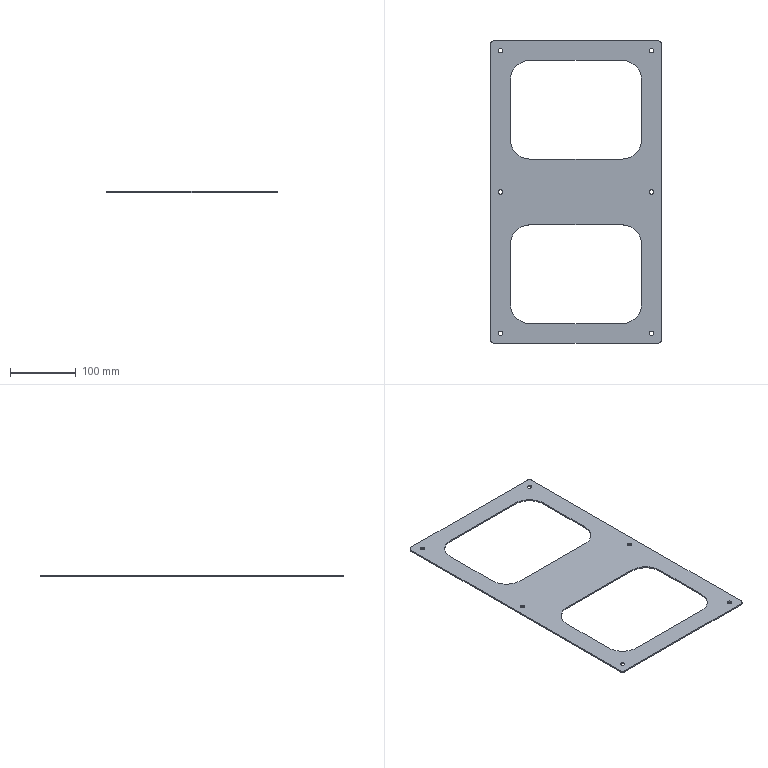Part | SolidWorks | features ICE 2, Extrusion 1, Fillet 1 | 1 solid | 38 faces | box 260 x 460 x 2 mm | volume 121786 mm3 | cylinder 24 | plane 14 | commonest cylinder face diameters 7 x12 60 x8 10 x4
STEP:
#1=CARTESIAN_POINT('',(18.5,-230.,2.));
#2=VERTEX_POINT('',#1);
#3=CARTESIAN_POINT('',(11.5,-230.,2.));
#4=VERTEX_POINT('',#3);
#5=CARTESIAN_POINT('',(15.,-230.,2.));
#6=DIRECTION('',(0.,0.,-1.));
#7=DIRECTION('',(-1.,0.,0.));
#8=AXIS2_PLACEMENT_3D('',#5,#6,#7);
#9=CIRCLE('',#8,3.5);
#10=EDGE_CURVE('',#2,#4,#9,.T.);
#11=ORIENTED_EDGE('',*,*,#10,.F.);
#12=CARTESIAN_POINT('',(18.5,-230.,0.));
#13=VERTEX_POINT('',#12);
#14=CARTESIAN_POINT('',(18.5,-230.,2.));
#15=DIRECTION('',(0.,0.,-1.));
#16=VECTOR('',#15,1000.);
#17=LINE('',#14,#16);
#18=EDGE_CURVE('',#2,#13,#17,.T.);
#19=ORIENTED_EDGE('',*,*,#18,.T.);
#20=CARTESIAN_POINT('',(11.5,-230.,0.));
#21=VERTEX_POINT('',#20);
#22=CARTESIAN_POINT('',(15.,-230.,0.));
#23=DIRECTION('',(0.,0.,-1.));
#24=DIRECTION('',(-1.,0.,0.));
#25=AXIS2_PLACEMENT_3D('',#22,#23,#24);
#26=CIRCLE('',#25,3.5);
#27=EDGE_CURVE('',#13,#21,#26,.T.);
#28=ORIENTED_EDGE('',*,*,#27,.T.);
#29=CARTESIAN_POINT('',(11.5,-230.,2.));
#30=DIRECTION('',(0.,0.,-1.));
#31=VECTOR('',#30,1000.);
#32=LINE('',#29,#31);
#33=EDGE_CURVE('',#4,#21,#32,.T.);
#34=ORIENTED_EDGE('',*,*,#33,.F.);
#35=EDGE_LOOP('',(#11,#19,#28,#34));
#36=FACE_OUTER_BOUND('',#35,.T.);
#37=CARTESIAN_POINT('',(15.,-230.,2.));
#38=DIRECTION('',(0.,0.,-1.));
#39=DIRECTION('',(-1.,0.,0.));
#40=AXIS2_PLACEMENT_3D('',#37,#38,#39);
#41=CYLINDRICAL_SURFACE('',#40,3.5);
#42=ADVANCED_FACE('',(#36),#41,.F.);
#43=CARTESIAN_POINT('',(248.5,-230.,2.));
#44=VERTEX_POINT('',#43);
#45=CARTESIAN_POINT('',(241.5,-230.,2.));
#46=VERTEX_POINT('',#45);
#47=CARTESIAN_POINT('',(245.,-230.,2.));
#48=DIRECTION('',(0.,0.,-1.));
#49=DIRECTION('',(-1.,0.,0.));
#50=AXIS2_PLACEMENT_3D('',#47,#48,#49);
#51=CIRCLE('',#50,3.5);
#52=EDGE_CURVE('',#44,#46,#51,.T.);
#53=ORIENTED_EDGE('',*,*,#52,.F.);
#54=CARTESIAN_POINT('',(248.5,-230.,0.));
#55=VERTEX_POINT('',#54);
#56=CARTESIAN_POINT('',(248.5,-230.,2.));
#57=DIRECTION('',(0.,0.,-1.));
#58=VECTOR('',#57,1000.);
#59=LINE('',#56,#58);
#60=EDGE_CURVE('',#44,#55,#59,.T.);
#61=ORIENTED_EDGE('',*,*,#60,.T.);
#62=CARTESIAN_POINT('',(241.5,-230.,0.));
#63=VERTEX_POINT('',#62);
#64=CARTESIAN_POINT('',(245.,-230.,0.));
#65=DIRECTION('',(0.,0.,-1.));
#66=DIRECTION('',(-1.,0.,0.));
#67=AXIS2_PLACEMENT_3D('',#64,#65,#66);
#68=CIRCLE('',#67,3.5);
#69=EDGE_CURVE('',#55,#63,#68,.T.);
#70=ORIENTED_EDGE('',*,*,#69,.T.);
#71=CARTESIAN_POINT('',(241.5,-230.,2.));
#72=DIRECTION('',(0.,0.,-1.));
#73=VECTOR('',#72,1000.);
#74=LINE('',#71,#73);
#75=EDGE_CURVE('',#46,#63,#74,.T.);
#76=ORIENTED_EDGE('',*,*,#75,.F.);
#77=EDGE_LOOP('',(#53,#61,#70,#76));
#78=FACE_OUTER_BOUND('',#77,.T.);
#79=CARTESIAN_POINT('',(245.,-230.,2.));
#80=DIRECTION('',(0.,0.,-1.));
#81=DIRECTION('',(-1.,0.,0.));
#82=AXIS2_PLACEMENT_3D('',#79,#80,#81);
#83=CYLINDRICAL_SURFACE('',#82,3.5);
#84=ADVANCED_FACE('',(#78),#83,.F.);
#85=CARTESIAN_POINT('',(18.5,-15.,2.));
#86=VERTEX_POINT('',#85);
#87=CARTESIAN_POINT('',(11.5,-15.,2.));
#88=VERTEX_POINT('',#87);
#89=CARTESIAN_POINT('',(15.,-15.,2.));
#90=DIRECTION('',(0.,0.,-1.));
#91=DIRECTION('',(-1.,0.,0.));
#92=AXIS2_PLACEMENT_3D('',#89,#90,#91);
#93=CIRCLE('',#92,3.5);
#94=EDGE_CURVE('',#86,#88,#93,.T.);
#95=ORIENTED_EDGE('',*,*,#94,.F.);
#96=CARTESIAN_POINT('',(18.5,-15.,0.));
#97=VERTEX_POINT('',#96);
#98=CARTESIAN_POINT('',(18.5,-15.,2.));
#99=DIRECTION('',(0.,0.,-1.));
#100=VECTOR('',#99,1000.);
#101=LINE('',#98,#100);
#102=EDGE_CURVE('',#86,#97,#101,.T.);
#103=ORIENTED_EDGE('',*,*,#102,.T.);
#104=CARTESIAN_POINT('',(11.5,-15.,0.));
#105=VERTEX_POINT('',#104);
#106=CARTESIAN_POINT('',(15.,-15.,0.));
#107=DIRECTION('',(0.,0.,-1.));
#108=DIRECTION('',(-1.,0.,0.));
#109=AXIS2_PLACEMENT_3D('',#106,#107,#108);
#110=CIRCLE('',#109,3.5);
#111=EDGE_CURVE('',#97,#105,#110,.T.);
#112=ORIENTED_EDGE('',*,*,#111,.T.);
#113=CARTESIAN_POINT('',(11.5,-15.,2.));
#114=DIRECTION('',(0.,0.,-1.));
#115=VECTOR('',#114,1000.);
#116=LINE('',#113,#115);
#117=EDGE_CURVE('',#88,#105,#116,.T.);
#118=ORIENTED_EDGE('',*,*,#117,.F.);
#119=EDGE_LOOP('',(#95,#103,#112,#118));
#120=FACE_OUTER_BOUND('',#119,.T.);
#121=CARTESIAN_POINT('',(15.,-15.,2.));
#122=DIRECTION('',(0.,0.,-1.));
#123=DIRECTION('',(-1.,0.,0.));
#124=AXIS2_PLACEMENT_3D('',#121,#122,#123);
#125=CYLINDRICAL_SURFACE('',#124,3.5);
#126=ADVANCED_FACE('',(#120),#125,.F.);
#127=CARTESIAN_POINT('',(248.5,-15.,2.));
#128=VERTEX_POINT('',#127);
#129=CARTESIAN_POINT('',(241.5,-15.,2.));
#130=VERTEX_POINT('',#129);
#131=CARTESIAN_POINT('',(245.,-15.,2.));
#132=DIRECTION('',(0.,0.,-1.));
#133=DIRECTION('',(-1.,0.,0.));
#134=AXIS2_PLACEMENT_3D('',#131,#132,#133);
#135=CIRCLE('',#134,3.5);
#136=EDGE_CURVE('',#128,#130,#135,.T.);
#137=ORIENTED_EDGE('',*,*,#136,.F.);
#138=CARTESIAN_POINT('',(248.5,-15.,0.));
#139=VERTEX_POINT('',#138);
#140=CARTESIAN_POINT('',(248.5,-15.,2.));
#141=DIRECTION('',(0.,0.,-1.));
#142=VECTOR('',#141,1000.);
#143=LINE('',#140,#142);
#144=EDGE_CURVE('',#128,#139,#143,.T.);
#145=ORIENTED_EDGE('',*,*,#144,.T.);
#146=CARTESIAN_POINT('',(241.5,-15.,0.));
#147=VERTEX_POINT('',#146);
#148=CARTESIAN_POINT('',(245.,-15.,0.));
#149=DIRECTION('',(0.,0.,-1.));
#150=DIRECTION('',(-1.,0.,0.));
#151=AXIS2_PLACEMENT_3D('',#148,#149,#150);
#152=CIRCLE('',#151,3.5);
#153=EDGE_CURVE('',#139,#147,#152,.T.);
#154=ORIENTED_EDGE('',*,*,#153,.T.);
#155=CARTESIAN_POINT('',(241.5,-15.,2.));
#156=DIRECTION('',(0.,0.,-1.));
#157=VECTOR('',#156,1000.);
#158=LINE('',#155,#157);
#159=EDGE_CURVE('',#130,#147,#158,.T.);
#160=ORIENTED_EDGE('',*,*,#159,.F.);
#161=EDGE_LOOP('',(#137,#145,#154,#160));
#162=FACE_OUTER_BOUND('',#161,.T.);
#163=CARTESIAN_POINT('',(245.,-15.,2.));
#164=DIRECTION('',(0.,0.,-1.));
#165=DIRECTION('',(-1.,0.,0.));
#166=AXIS2_PLACEMENT_3D('',#163,#164,#165);
#167=CYLINDRICAL_SURFACE('',#166,3.5);
#168=ADVANCED_FACE('',(#162),#167,.F.);
#169=CARTESIAN_POINT('',(18.5,-445.,2.));
#170=VERTEX_POINT('',#169);
#171=CARTESIAN_POINT('',(11.5,-445.,2.));
#172=VERTEX_POINT('',#171);
#173=CARTESIAN_POINT('',(15.,-445.,2.));
#174=DIRECTION('',(0.,0.,-1.));
#175=DIRECTION('',(-1.,0.,0.));
#176=AXIS2_PLACEMENT_3D('',#173,#174,#175);
#177=CIRCLE('',#176,3.5);
#178=EDGE_CURVE('',#170,#172,#177,.T.);
#179=ORIENTED_EDGE('',*,*,#178,.F.);
#180=CARTESIAN_POINT('',(18.5,-445.,0.));
#181=VERTEX_POINT('',#180);
#182=CARTESIAN_POINT('',(18.5,-445.,2.));
#183=DIRECTION('',(0.,0.,-1.));
#184=VECTOR('',#183,1000.);
#185=LINE('',#182,#184);
#186=EDGE_CURVE('',#170,#181,#185,.T.);
#187=ORIENTED_EDGE('',*,*,#186,.T.);
#188=CARTESIAN_POINT('',(11.5,-445.,0.));
#189=VERTEX_POINT('',#188);
#190=CARTESIAN_POINT('',(15.,-445.,0.));
#191=DIRECTION('',(0.,0.,-1.));
#192=DIRECTION('',(-1.,0.,0.));
#193=AXIS2_PLACEMENT_3D('',#190,#191,#192);
#194=CIRCLE('',#193,3.5);
#195=EDGE_CURVE('',#181,#189,#194,.T.);
#196=ORIENTED_EDGE('',*,*,#195,.T.);
#197=CARTESIAN_POINT('',(11.5,-445.,2.));
#198=DIRECTION('',(0.,0.,-1.));
#199=VECTOR('',#198,1000.);
#200=LINE('',#197,#199);
#201=EDGE_CURVE('',#172,#189,#200,.T.);
#202=ORIENTED_EDGE('',*,*,#201,.F.);
#203=EDGE_LOOP('',(#179,#187,#196,#202));
#204=FACE_OUTER_BOUND('',#203,.T.);
#205=CARTESIAN_POINT('',(15.,-445.,2.));
#206=DIRECTION('',(0.,0.,-1.));
#207=DIRECTION('',(-1.,0.,0.));
#208=AXIS2_PLACEMENT_3D('',#205,#206,#207);
#209=CYLINDRICAL_SURFACE('',#208,3.5);
#210=ADVANCED_FACE('',(#204),#209,.F.);
#211=CARTESIAN_POINT('',(248.5,-445.,2.));
#212=VERTEX_POINT('',#211);
#213=CARTESIAN_POINT('',(241.5,-445.,2.));
#214=VERTEX_POINT('',#213);
#215=CARTESIAN_POINT('',(245.,-445.,2.));
#216=DIRECTION('',(0.,0.,-1.));
#217=DIRECTION('',(-1.,0.,0.));
#218=AXIS2_PLACEMENT_3D('',#215,#216,#217);
#219=CIRCLE('',#218,3.5);
#220=EDGE_CURVE('',#212,#214,#219,.T.);
#221=ORIENTED_EDGE('',*,*,#220,.F.);
#222=CARTESIAN_POINT('',(248.5,-445.,0.));
#223=VERTEX_POINT('',#222);
#224=CARTESIAN_POINT('',(248.5,-445.,2.));
#225=DIRECTION('',(0.,0.,-1.));
#226=VECTOR('',#225,1000.);
#227=LINE('',#224,#226);
#228=EDGE_CURVE('',#212,#223,#227,.T.);
#229=ORIENTED_EDGE('',*,*,#228,.T.);
#230=CARTESIAN_POINT('',(241.5,-445.,0.));
#231=VERTEX_POINT('',#230);
#232=CARTESIAN_POINT('',(245.,-445.,0.));
#233=DIRECTION('',(0.,0.,-1.));
#234=DIRECTION('',(-1.,0.,0.));
#235=AXIS2_PLACEMENT_3D('',#232,#233,#234);
#236=CIRCLE('',#235,3.5);
#237=EDGE_CURVE('',#223,#231,#236,.T.);
#238=ORIENTED_EDGE('',*,*,#237,.T.);
#239=CARTESIAN_POINT('',(241.5,-445.,2.));
#240=DIRECTION('',(0.,0.,-1.));
#241=VECTOR('',#240,1000.);
#242=LINE('',#239,#241);
#243=EDGE_CURVE('',#214,#231,#242,.T.);
#244=ORIENTED_EDGE('',*,*,#243,.F.);
#245=EDGE_LOOP('',(#221,#229,#238,#244));
#246=FACE_OUTER_BOUND('',#245,.T.);
#247=CARTESIAN_POINT('',(245.,-445.,2.));
#248=DIRECTION('',(0.,0.,-1.));
#249=DIRECTION('',(-1.,0.,0.));
#250=AXIS2_PLACEMENT_3D('',#247,#248,#249);
#251=CYLINDRICAL_SURFACE('',#250,3.5);
#252=ADVANCED_FACE('',(#246),#251,.F.);
#253=CARTESIAN_POINT('',(0.,-5.,0.));
#254=VERTEX_POINT('',#253);
#255=CARTESIAN_POINT('',(0.,-455.,0.));
#256=VERTEX_POINT('',#255);
#257=CARTESIAN_POINT('',(0.,0.,0.));
#258=DIRECTION('',(0.,-1.,0.));
#259=VECTOR('',#258,1000.);
#260=LINE('',#257,#259);
#261=EDGE_CURVE('',#254,#256,#260,.T.);
#262=ORIENTED_EDGE('',*,*,#261,.T.);
#263=CARTESIAN_POINT('',(0.,-455.,2.));
#264=VERTEX_POINT('',#263);
#265=CARTESIAN_POINT('',(0.,-455.,2.));
#266=DIRECTION('',(0.,0.,1.));
#267=VECTOR('',#266,1000.);
#268=LINE('',#265,#267);
#269=EDGE_CURVE('',#256,#264,#268,.T.);
#270=ORIENTED_EDGE('',*,*,#269,.T.);
#271=CARTESIAN_POINT('',(0.,-5.,2.));
#272=VERTEX_POINT('',#271);
#273=CARTESIAN_POINT('',(0.,0.,2.));
#274=DIRECTION('',(0.,-1.,0.));
#275=VECTOR('',#274,1000.);
#276=LINE('',#273,#275);
#277=EDGE_CURVE('',#272,#264,#276,.T.);
#278=ORIENTED_EDGE('',*,*,#277,.F.);
#279=CARTESIAN_POINT('',(0.,-5.,2.));
#280=DIRECTION('',(0.,0.,-1.));
#281=VECTOR('',#280,1000.);
#282=LINE('',#279,#281);
#283=EDGE_CURVE('',#272,#254,#282,.T.);
#284=ORIENTED_EDGE('',*,*,#283,.T.);
#285=EDGE_LOOP('',(#262,#270,#278,#284));
#286=FACE_OUTER_BOUND('',#285,.T.);
#287=CARTESIAN_POINT('',(0.,0.,2.));
#288=DIRECTION('',(1.,0.,0.));
#289=DIRECTION('',(0.,1.,0.));
#290=AXIS2_PLACEMENT_3D('',#287,#288,#289);
#291=PLANE('',#290);
#292=ADVANCED_FACE('',(#286),#291,.F.);
#293=CARTESIAN_POINT('',(5.,-460.,2.));
#294=VERTEX_POINT('',#293);
#295=CARTESIAN_POINT('',(255.,-460.,2.));
#296=VERTEX_POINT('',#295);
#297=CARTESIAN_POINT('',(0.,-460.,2.));
#298=DIRECTION('',(1.,0.,0.));
#299=VECTOR('',#298,1000.);
#300=LINE('',#297,#299);
#301=EDGE_CURVE('',#294,#296,#300,.T.);
#302=ORIENTED_EDGE('',*,*,#301,.F.);
#303=CARTESIAN_POINT('',(5.,-460.,0.));
#304=VERTEX_POINT('',#303);
#305=CARTESIAN_POINT('',(5.,-460.,2.));
#306=DIRECTION('',(0.,0.,-1.));
#307=VECTOR('',#306,1000.);
#308=LINE('',#305,#307);
#309=EDGE_CURVE('',#294,#304,#308,.T.);
#310=ORIENTED_EDGE('',*,*,#309,.T.);
#311=CARTESIAN_POINT('',(255.,-460.,0.));
#312=VERTEX_POINT('',#311);
#313=CARTESIAN_POINT('',(0.,-460.,0.));
#314=DIRECTION('',(1.,0.,0.));
#315=VECTOR('',#314,1000.);
#316=LINE('',#313,#315);
#317=EDGE_CURVE('',#304,#312,#316,.T.);
#318=ORIENTED_EDGE('',*,*,#317,.T.);
#319=CARTESIAN_POINT('',(255.,-460.,2.));
#320=DIRECTION('',(0.,0.,1.));
#321=VECTOR('',#320,1000.);
#322=LINE('',#319,#321);
#323=EDGE_CURVE('',#312,#296,#322,.T.);
#324=ORIENTED_EDGE('',*,*,#323,.T.);
#325=EDGE_LOOP('',(#302,#310,#318,#324));
#326=FACE_OUTER_BOUND('',#325,.T.);
#327=CARTESIAN_POINT('',(0.,-460.,2.));
#328=DIRECTION('',(0.,1.,0.));
#329=DIRECTION('',(0.,0.,1.));
#330=AXIS2_PLACEMENT_3D('',#327,#328,#329);
#331=PLANE('',#330);
#332=ADVANCED_FACE('',(#326),#331,.F.);
#333=CARTESIAN_POINT('',(260.,-455.,2.));
#334=VERTEX_POINT('',#333);
#335=CARTESIAN_POINT('',(260.,-5.,2.));
#336=VERTEX_POINT('',#335);
#337=CARTESIAN_POINT('',(260.,0.,2.));
#338=DIRECTION('',(0.,1.,0.));
#339=VECTOR('',#338,1000.);
#340=LINE('',#337,#339);
#341=EDGE_CURVE('',#334,#336,#340,.T.);
#342=ORIENTED_EDGE('',*,*,#341,.F.);
#343=CARTESIAN_POINT('',(260.,-455.,0.));
#344=VERTEX_POINT('',#343);
#345=CARTESIAN_POINT('',(260.,-455.,2.));
#346=DIRECTION('',(0.,0.,-1.));
#347=VECTOR('',#346,1000.);
#348=LINE('',#345,#347);
#349=EDGE_CURVE('',#334,#344,#348,.T.);
#350=ORIENTED_EDGE('',*,*,#349,.T.);
#351=CARTESIAN_POINT('',(260.,-5.,0.));
#352=VERTEX_POINT('',#351);
#353=CARTESIAN_POINT('',(260.,0.,0.));
#354=DIRECTION('',(0.,1.,0.));
#355=VECTOR('',#354,1000.);
#356=LINE('',#353,#355);
#357=EDGE_CURVE('',#344,#352,#356,.T.);
#358=ORIENTED_EDGE('',*,*,#357,.T.);
#359=CARTESIAN_POINT('',(260.,-5.,2.));
#360=DIRECTION('',(0.,0.,1.));
#361=VECTOR('',#360,1000.);
#362=LINE('',#359,#361);
#363=EDGE_CURVE('',#352,#336,#362,.T.);
#364=ORIENTED_EDGE('',*,*,#363,.T.);
#365=EDGE_LOOP('',(#342,#350,#358,#364));
#366=FACE_OUTER_BOUND('',#365,.T.);
#367=CARTESIAN_POINT('',(260.,0.,2.));
#368=DIRECTION('',(-1.,0.,0.));
#369=DIRECTION('',(0.,-1.,0.));
#370=AXIS2_PLACEMENT_3D('',#367,#368,#369);
#371=PLANE('',#370);
#372=ADVANCED_FACE('',(#366),#371,.F.);
#373=CARTESIAN_POINT('',(255.,0.,2.));
#374=VERTEX_POINT('',#373);
#375=CARTESIAN_POINT('',(5.,0.,2.));
#376=VERTEX_POINT('',#375);
#377=CARTESIAN_POINT('',(0.,0.,2.));
#378=DIRECTION('',(-1.,0.,0.));
#379=VECTOR('',#378,1000.);
#380=LINE('',#377,#379);
#381=EDGE_CURVE('',#374,#376,#380,.T.);
#382=ORIENTED_EDGE('',*,*,#381,.F.);
#383=CARTESIAN_POINT('',(255.,0.,0.));
#384=VERTEX_POINT('',#383);
#385=CARTESIAN_POINT('',(255.,0.,2.));
#386=DIRECTION('',(0.,0.,-1.));
#387=VECTOR('',#386,1000.);
#388=LINE('',#385,#387);
#389=EDGE_CURVE('',#374,#384,#388,.T.);
#390=ORIENTED_EDGE('',*,*,#389,.T.);
#391=CARTESIAN_POINT('',(5.,0.,0.));
#392=VERTEX_POINT('',#391);
#393=CARTESIAN_POINT('',(0.,0.,0.));
#394=DIRECTION('',(-1.,0.,0.));
#395=VECTOR('',#394,1000.);
#396=LINE('',#393,#395);
#397=EDGE_CURVE('',#384,#392,#396,.T.);
#398=ORIENTED_EDGE('',*,*,#397,.T.);
#399=CARTESIAN_POINT('',(5.,0.,2.));
#400=DIRECTION('',(0.,0.,1.));
#401=VECTOR('',#400,1000.);
#402=LINE('',#399,#401);
#403=EDGE_CURVE('',#392,#376,#402,.T.);
#404=ORIENTED_EDGE('',*,*,#403,.T.);
#405=EDGE_LOOP('',(#382,#390,#398,#404));
#406=FACE_OUTER_BOUND('',#405,.T.);
#407=CARTESIAN_POINT('',(0.,0.,2.));
#408=DIRECTION('',(0.,-1.,0.));
#409=DIRECTION('',(0.,0.,-1.));
#410=AXIS2_PLACEMENT_3D('',#407,#408,#409);
#411=PLANE('',#410);
#412=ADVANCED_FACE('',(#406),#411,.F.);
#413=CARTESIAN_POINT('',(30.,-310.,2.));
#414=VERTEX_POINT('',#413);
#415=CARTESIAN_POINT('',(60.,-280.,2.));
#416=VERTEX_POINT('',#415);
#417=CARTESIAN_POINT('',(60.,-310.,2.));
#418=DIRECTION('',(0.,0.,-1.));
#419=DIRECTION('',(-1.,0.,0.));
#420=AXIS2_PLACEMENT_3D('',#417,#418,#419);
#421=CIRCLE('',#420,30.);
#422=EDGE_CURVE('',#414,#416,#421,.T.);
#423=ORIENTED_EDGE('',*,*,#422,.T.);
#424=CARTESIAN_POINT('',(200.,-280.,2.));
#425=VERTEX_POINT('',#424);
#426=CARTESIAN_POINT('',(60.,-280.,2.));
#427=DIRECTION('',(1.,0.,0.));
#428=VECTOR('',#427,1000.);
#429=LINE('',#426,#428);
#430=EDGE_CURVE('',#416,#425,#429,.T.);
#431=ORIENTED_EDGE('',*,*,#430,.T.);
#432=CARTESIAN_POINT('',(230.,-310.,2.));
#433=VERTEX_POINT('',#432);
#434=CARTESIAN_POINT('',(200.,-310.,2.));
#435=DIRECTION('',(0.,0.,-1.));
#436=DIRECTION('',(-1.,0.,0.));
#437=AXIS2_PLACEMENT_3D('',#434,#435,#436);
#438=CIRCLE('',#437,30.);
#439=EDGE_CURVE('',#425,#433,#438,.T.);
#440=ORIENTED_EDGE('',*,*,#439,.T.);
#441=CARTESIAN_POINT('',(230.,-400.,2.));
#442=VERTEX_POINT('',#441);
#443=CARTESIAN_POINT('',(230.,-400.,2.));
#444=DIRECTION('',(0.,-1.,0.));
#445=VECTOR('',#444,1000.);
#446=LINE('',#443,#445);
#447=EDGE_CURVE('',#433,#442,#446,.T.);
#448=ORIENTED_EDGE('',*,*,#447,.T.);
#449=CARTESIAN_POINT('',(200.,-430.,2.));
#450=VERTEX_POINT('',#449);
#451=CARTESIAN_POINT('',(200.,-400.,2.));
#452=DIRECTION('',(0.,0.,-1.));
#453=DIRECTION('',(-1.,0.,0.));
#454=AXIS2_PLACEMENT_3D('',#451,#452,#453);
#455=CIRCLE('',#454,30.);
#456=EDGE_CURVE('',#442,#450,#455,.T.);
#457=ORIENTED_EDGE('',*,*,#456,.T.);
#458=CARTESIAN_POINT('',(60.,-430.,2.));
#459=VERTEX_POINT('',#458);
#460=CARTESIAN_POINT('',(60.,-430.,2.));
#461=DIRECTION('',(-1.,0.,0.));
#462=VECTOR('',#461,1000.);
#463=LINE('',#460,#462);
#464=EDGE_CURVE('',#450,#459,#463,.T.);
#465=ORIENTED_EDGE('',*,*,#464,.T.);
#466=CARTESIAN_POINT('',(30.,-400.,2.));
#467=VERTEX_POINT('',#466);
#468=CARTESIAN_POINT('',(60.,-400.,2.));
#469=DIRECTION('',(0.,0.,-1.));
#470=DIRECTION('',(-1.,0.,0.));
#471=AXIS2_PLACEMENT_3D('',#468,#469,#470);
#472=CIRCLE('',#471,30.);
#473=EDGE_CURVE('',#459,#467,#472,.T.);
#474=ORIENTED_EDGE('',*,*,#473,.T.);
#475=CARTESIAN_POINT('',(30.,-400.,2.));
#476=DIRECTION('',(0.,1.,0.));
#477=VECTOR('',#476,1000.);
#478=LINE('',#475,#477);
#479=EDGE_CURVE('',#467,#414,#478,.T.);
#480=ORIENTED_EDGE('',*,*,#479,.T.);
#481=EDGE_LOOP('',(#423,#431,#440,#448,#457,#465,#474,#480));
#482=FACE_BOUND('',#481,.T.);
#483=CARTESIAN_POINT('',(30.,-60.,2.));
#484=VERTEX_POINT('',#483);
#485=CARTESIAN_POINT('',(60.,-30.,2.));
#486=VERTEX_POINT('',#485);
#487=CARTESIAN_POINT('',(60.,-60.,2.));
#488=DIRECTION('',(0.,0.,-1.));
#489=DIRECTION('',(-1.,0.,0.));
#490=AXIS2_PLACEMENT_3D('',#487,#488,#489);
#491=CIRCLE('',#490,30.);
#492=EDGE_CURVE('',#484,#486,#491,.T.);
#493=ORIENTED_EDGE('',*,*,#492,.T.);
#494=CARTESIAN_POINT('',(200.,-30.,2.));
#495=VERTEX_POINT('',#494);
#496=CARTESIAN_POINT('',(60.,-30.,2.));
#497=DIRECTION('',(1.,0.,0.));
#498=VECTOR('',#497,1000.);
#499=LINE('',#496,#498);
#500=EDGE_CURVE('',#486,#495,#499,.T.);
#501=ORIENTED_EDGE('',*,*,#500,.T.);
#502=CARTESIAN_POINT('',(230.,-60.,2.));
#503=VERTEX_POINT('',#502);
#504=CARTESIAN_POINT('',(200.,-60.,2.));
#505=DIRECTION('',(0.,0.,-1.));
#506=DIRECTION('',(-1.,0.,0.));
#507=AXIS2_PLACEMENT_3D('',#504,#505,#506);
#508=CIRCLE('',#507,30.);
#509=EDGE_CURVE('',#495,#503,#508,.T.);
#510=ORIENTED_EDGE('',*,*,#509,.T.);
#511=CARTESIAN_POINT('',(230.,-150.,2.));
#512=VERTEX_POINT('',#511);
#513=CARTESIAN_POINT('',(230.,-150.,2.));
#514=DIRECTION('',(0.,-1.,0.));
#515=VECTOR('',#514,1000.);
#516=LINE('',#513,#515);
#517=EDGE_CURVE('',#503,#512,#516,.T.);
#518=ORIENTED_EDGE('',*,*,#517,.T.);
#519=CARTESIAN_POINT('',(200.,-180.,2.));
#520=VERTEX_POINT('',#519);
#521=CARTESIAN_POINT('',(200.,-150.,2.));
#522=DIRECTION('',(0.,0.,-1.));
#523=DIRECTION('',(-1.,0.,0.));
#524=AXIS2_PLACEMENT_3D('',#521,#522,#523);
#525=CIRCLE('',#524,30.);
#526=EDGE_CURVE('',#512,#520,#525,.T.);
#527=ORIENTED_EDGE('',*,*,#526,.T.);
#528=CARTESIAN_POINT('',(60.,-180.,2.));
#529=VERTEX_POINT('',#528);
#530=CARTESIAN_POINT('',(60.,-180.,2.));
#531=DIRECTION('',(-1.,0.,0.));
#532=VECTOR('',#531,1000.);
#533=LINE('',#530,#532);
#534=EDGE_CURVE('',#520,#529,#533,.T.);
#535=ORIENTED_EDGE('',*,*,#534,.T.);
#536=CARTESIAN_POINT('',(30.,-150.,2.));
#537=VERTEX_POINT('',#536);
#538=CARTESIAN_POINT('',(60.,-150.,2.));
#539=DIRECTION('',(0.,0.,-1.));
#540=DIRECTION('',(-1.,0.,0.));
#541=AXIS2_PLACEMENT_3D('',#538,#539,#540);
#542=CIRCLE('',#541,30.);
#543=EDGE_CURVE('',#529,#537,#542,.T.);
#544=ORIENTED_EDGE('',*,*,#543,.T.);
#545=CARTESIAN_POINT('',(30.,-150.,2.));
#546=DIRECTION('',(0.,1.,0.));
#547=VECTOR('',#546,1000.);
#548=LINE('',#545,#547);
#549=EDGE_CURVE('',#537,#484,#548,.T.);
#550=ORIENTED_EDGE('',*,*,#549,.T.);
#551=EDGE_LOOP('',(#493,#501,#510,#518,#527,#535,#544,#550));
#552=FACE_BOUND('',#551,.T.);
#553=CARTESIAN_POINT('',(15.,-230.,2.));
#554=DIRECTION('',(0.,0.,-1.));
#555=DIRECTION('',(-1.,0.,0.));
#556=AXIS2_PLACEMENT_3D('',#553,#554,#555);
#557=CIRCLE('',#556,3.5);
#558=EDGE_CURVE('',#4,#2,#557,.T.);
#559=ORIENTED_EDGE('',*,*,#558,.T.);
#560=ORIENTED_EDGE('',*,*,#10,.T.);
#561=EDGE_LOOP('',(#559,#560));
#562=FACE_BOUND('',#561,.T.);
#563=CARTESIAN_POINT('',(245.,-230.,2.));
#564=DIRECTION('',(0.,0.,-1.));
#565=DIRECTION('',(-1.,0.,0.));
#566=AXIS2_PLACEMENT_3D('',#563,#564,#565);
#567=CIRCLE('',#566,3.5);
#568=EDGE_CURVE('',#46,#44,#567,.T.);
#569=ORIENTED_EDGE('',*,*,#568,.T.);
#570=ORIENTED_EDGE('',*,*,#52,.T.);
#571=EDGE_LOOP('',(#569,#570));
#572=FACE_BOUND('',#571,.T.);
#573=CARTESIAN_POINT('',(15.,-15.,2.));
#574=DIRECTION('',(0.,0.,-1.));
#575=DIRECTION('',(-1.,0.,0.));
#576=AXIS2_PLACEMENT_3D('',#573,#574,#575);
#577=CIRCLE('',#576,3.5);
#578=EDGE_CURVE('',#88,#86,#577,.T.);
#579=ORIENTED_EDGE('',*,*,#578,.T.);
#580=ORIENTED_EDGE('',*,*,#94,.T.);
#581=EDGE_LOOP('',(#579,#580));
#582=FACE_BOUND('',#581,.T.);
#583=CARTESIAN_POINT('',(245.,-15.,2.));
#584=DIRECTION('',(0.,0.,-1.));
#585=DIRECTION('',(-1.,0.,0.));
#586=AXIS2_PLACEMENT_3D('',#583,#584,#585);
#587=CIRCLE('',#586,3.5);
#588=EDGE_CURVE('',#130,#128,#587,.T.);
#589=ORIENTED_EDGE('',*,*,#588,.T.);
#590=ORIENTED_EDGE('',*,*,#136,.T.);
#591=EDGE_LOOP('',(#589,#590));
#592=FACE_BOUND('',#591,.T.);
#593=CARTESIAN_POINT('',(15.,-445.,2.));
#594=DIRECTION('',(0.,0.,-1.));
#595=DIRECTION('',(-1.,0.,0.));
#596=AXIS2_PLACEMENT_3D('',#593,#594,#595);
#597=CIRCLE('',#596,3.5);
#598=EDGE_CURVE('',#172,#170,#597,.T.);
#599=ORIENTED_EDGE('',*,*,#598,.T.);
#600=ORIENTED_EDGE('',*,*,#178,.T.);
#601=EDGE_LOOP('',(#599,#600));
#602=FACE_BOUND('',#601,.T.);
#603=CARTESIAN_POINT('',(245.,-445.,2.));
#604=DIRECTION('',(0.,0.,-1.));
#605=DIRECTION('',(-1.,0.,0.));
#606=AXIS2_PLACEMENT_3D('',#603,#604,#605);
#607=CIRCLE('',#606,3.5);
#608=EDGE_CURVE('',#214,#212,#607,.T.);
#609=ORIENTED_EDGE('',*,*,#608,.T.);
#610=ORIENTED_EDGE('',*,*,#220,.T.);
#611=EDGE_LOOP('',(#609,#610));
#612=FACE_BOUND('',#611,.T.);
#613=ORIENTED_EDGE('',*,*,#277,.T.);
#614=CARTESIAN_POINT('',(5.,-455.,2.));
#615=DIRECTION('',(0.,0.,1.));
#616=DIRECTION('',(1.,0.,0.));
#617=AXIS2_PLACEMENT_3D('',#614,#615,#616);
#618=CIRCLE('',#617,5.);
#619=EDGE_CURVE('',#264,#294,#618,.T.);
#620=ORIENTED_EDGE('',*,*,#619,.T.);
#621=ORIENTED_EDGE('',*,*,#301,.T.);
#622=CARTESIAN_POINT('',(255.,-455.,2.));
#623=DIRECTION('',(0.,0.,1.));
#624=DIRECTION('',(1.,0.,0.));
#625=AXIS2_PLACEMENT_3D('',#622,#623,#624);
#626=CIRCLE('',#625,5.);
#627=EDGE_CURVE('',#296,#334,#626,.T.);
#628=ORIENTED_EDGE('',*,*,#627,.T.);
#629=ORIENTED_EDGE('',*,*,#341,.T.);
#630=CARTESIAN_POINT('',(255.,-5.,2.));
#631=DIRECTION('',(0.,0.,1.));
#632=DIRECTION('',(1.,0.,0.));
#633=AXIS2_PLACEMENT_3D('',#630,#631,#632);
#634=CIRCLE('',#633,5.);
#635=EDGE_CURVE('',#336,#374,#634,.T.);
#636=ORIENTED_EDGE('',*,*,#635,.T.);
#637=ORIENTED_EDGE('',*,*,#381,.T.);
#638=CARTESIAN_POINT('',(5.,-5.,2.));
#639=DIRECTION('',(0.,0.,1.));
#640=DIRECTION('',(1.,0.,0.));
#641=AXIS2_PLACEMENT_3D('',#638,#639,#640);
#642=CIRCLE('',#641,5.);
#643=EDGE_CURVE('',#376,#272,#642,.T.);
#644=ORIENTED_EDGE('',*,*,#643,.T.);
#645=EDGE_LOOP('',(#613,#620,#621,#628,#629,#636,#637,#644));
#646=FACE_OUTER_BOUND('',#645,.T.);
#647=CARTESIAN_POINT('',(0.,0.,2.));
#648=DIRECTION('',(0.,0.,1.));
#649=DIRECTION('',(1.,0.,0.));
#650=AXIS2_PLACEMENT_3D('',#647,#648,#649);
#651=PLANE('',#650);
#652=ADVANCED_FACE('',(#482,#552,#562,#572,#582,#592,#602,#612,#646),#651,.T.);
#653=CARTESIAN_POINT('',(60.,-280.,0.));
#654=VERTEX_POINT('',#653);
#655=CARTESIAN_POINT('',(200.,-280.,0.));
#656=VERTEX_POINT('',#655);
#657=CARTESIAN_POINT('',(60.,-280.,0.));
#658=DIRECTION('',(1.,0.,0.));
#659=VECTOR('',#658,1000.);
#660=LINE('',#657,#659);
#661=EDGE_CURVE('',#654,#656,#660,.T.);
#662=ORIENTED_EDGE('',*,*,#661,.F.);
#663=CARTESIAN_POINT('',(30.,-310.,0.));
#664=VERTEX_POINT('',#663);
#665=CARTESIAN_POINT('',(60.,-310.,0.));
#666=DIRECTION('',(0.,0.,-1.));
#667=DIRECTION('',(-1.,0.,0.));
#668=AXIS2_PLACEMENT_3D('',#665,#666,#667);
#669=CIRCLE('',#668,30.);
#670=EDGE_CURVE('',#664,#654,#669,.T.);
#671=ORIENTED_EDGE('',*,*,#670,.F.);
#672=CARTESIAN_POINT('',(30.,-400.,0.));
#673=VERTEX_POINT('',#672);
#674=CARTESIAN_POINT('',(30.,-400.,0.));
#675=DIRECTION('',(0.,1.,0.));
#676=VECTOR('',#675,1000.);
#677=LINE('',#674,#676);
#678=EDGE_CURVE('',#673,#664,#677,.T.);
#679=ORIENTED_EDGE('',*,*,#678,.F.);
#680=CARTESIAN_POINT('',(60.,-430.,0.));
#681=VERTEX_POINT('',#680);
#682=CARTESIAN_POINT('',(60.,-400.,0.));
#683=DIRECTION('',(0.,0.,-1.));
#684=DIRECTION('',(-1.,0.,0.));
#685=AXIS2_PLACEMENT_3D('',#682,#683,#684);
#686=CIRCLE('',#685,30.);
#687=EDGE_CURVE('',#681,#673,#686,.T.);
#688=ORIENTED_EDGE('',*,*,#687,.F.);
#689=CARTESIAN_POINT('',(200.,-430.,0.));
#690=VERTEX_POINT('',#689);
#691=CARTESIAN_POINT('',(60.,-430.,0.));
#692=DIRECTION('',(-1.,0.,0.));
#693=VECTOR('',#692,1000.);
#694=LINE('',#691,#693);
#695=EDGE_CURVE('',#690,#681,#694,.T.);
#696=ORIENTED_EDGE('',*,*,#695,.F.);
#697=CARTESIAN_POINT('',(230.,-400.,0.));
#698=VERTEX_POINT('',#697);
#699=CARTESIAN_POINT('',(200.,-400.,0.));
#700=DIRECTION('',(0.,0.,-1.));
#701=DIRECTION('',(-1.,0.,0.));
#702=AXIS2_PLACEMENT_3D('',#699,#700,#701);
#703=CIRCLE('',#702,30.);
#704=EDGE_CURVE('',#698,#690,#703,.T.);
#705=ORIENTED_EDGE('',*,*,#704,.F.);
#706=CARTESIAN_POINT('',(230.,-310.,0.));
#707=VERTEX_POINT('',#706);
#708=CARTESIAN_POINT('',(230.,-400.,0.));
#709=DIRECTION('',(0.,-1.,0.));
#710=VECTOR('',#709,1000.);
#711=LINE('',#708,#710);
#712=EDGE_CURVE('',#707,#698,#711,.T.);
#713=ORIENTED_EDGE('',*,*,#712,.F.);
#714=CARTESIAN_POINT('',(200.,-310.,0.));
#715=DIRECTION('',(0.,0.,-1.));
#716=DIRECTION('',(-1.,0.,0.));
#717=AXIS2_PLACEMENT_3D('',#714,#715,#716);
#718=CIRCLE('',#717,30.);
#719=EDGE_CURVE('',#656,#707,#718,.T.);
#720=ORIENTED_EDGE('',*,*,#719,.F.);
#721=EDGE_LOOP('',(#662,#671,#679,#688,#696,#705,#713,#720));
#722=FACE_BOUND('',#721,.T.);
#723=CARTESIAN_POINT('',(60.,-30.,0.));
#724=VERTEX_POINT('',#723);
#725=CARTESIAN_POINT('',(200.,-30.,0.));
#726=VERTEX_POINT('',#725);
#727=CARTESIAN_POINT('',(60.,-30.,0.));
#728=DIRECTION('',(1.,0.,0.));
#729=VECTOR('',#728,1000.);
#730=LINE('',#727,#729);
#731=EDGE_CURVE('',#724,#726,#730,.T.);
#732=ORIENTED_EDGE('',*,*,#731,.F.);
#733=CARTESIAN_POINT('',(30.,-60.,0.));
#734=VERTEX_POINT('',#733);
#735=CARTESIAN_POINT('',(60.,-60.,0.));
#736=DIRECTION('',(0.,0.,-1.));
#737=DIRECTION('',(-1.,0.,0.));
#738=AXIS2_PLACEMENT_3D('',#735,#736,#737);
#739=CIRCLE('',#738,30.);
#740=EDGE_CURVE('',#734,#724,#739,.T.);
#741=ORIENTED_EDGE('',*,*,#740,.F.);
#742=CARTESIAN_POINT('',(30.,-150.,0.));
#743=VERTEX_POINT('',#742);
#744=CARTESIAN_POINT('',(30.,-150.,0.));
#745=DIRECTION('',(0.,1.,0.));
#746=VECTOR('',#745,1000.);
#747=LINE('',#744,#746);
#748=EDGE_CURVE('',#743,#734,#747,.T.);
#749=ORIENTED_EDGE('',*,*,#748,.F.);
#750=CARTESIAN_POINT('',(60.,-180.,0.));
#751=VERTEX_POINT('',#750);
#752=CARTESIAN_POINT('',(60.,-150.,0.));
#753=DIRECTION('',(0.,0.,-1.));
#754=DIRECTION('',(-1.,0.,0.));
#755=AXIS2_PLACEMENT_3D('',#752,#753,#754);
#756=CIRCLE('',#755,30.);
#757=EDGE_CURVE('',#751,#743,#756,.T.);
#758=ORIENTED_EDGE('',*,*,#757,.F.);
#759=CARTESIAN_POINT('',(200.,-180.,0.));
#760=VERTEX_POINT('',#759);
#761=CARTESIAN_POINT('',(60.,-180.,0.));
#762=DIRECTION('',(-1.,0.,0.));
#763=VECTOR('',#762,1000.);
#764=LINE('',#761,#763);
#765=EDGE_CURVE('',#760,#751,#764,.T.);
#766=ORIENTED_EDGE('',*,*,#765,.F.);
#767=CARTESIAN_POINT('',(230.,-150.,0.));
#768=VERTEX_POINT('',#767);
#769=CARTESIAN_POINT('',(200.,-150.,0.));
#770=DIRECTION('',(0.,0.,-1.));
#771=DIRECTION('',(-1.,0.,0.));
#772=AXIS2_PLACEMENT_3D('',#769,#770,#771);
#773=CIRCLE('',#772,30.);
#774=EDGE_CURVE('',#768,#760,#773,.T.);
#775=ORIENTED_EDGE('',*,*,#774,.F.);
#776=CARTESIAN_POINT('',(230.,-60.,0.));
#777=VERTEX_POINT('',#776);
#778=CARTESIAN_POINT('',(230.,-150.,0.));
#779=DIRECTION('',(0.,-1.,0.));
#780=VECTOR('',#779,1000.);
#781=LINE('',#778,#780);
#782=EDGE_CURVE('',#777,#768,#781,.T.);
#783=ORIENTED_EDGE('',*,*,#782,.F.);
#784=CARTESIAN_POINT('',(200.,-60.,0.));
#785=DIRECTION('',(0.,0.,-1.));
#786=DIRECTION('',(-1.,0.,0.));
#787=AXIS2_PLACEMENT_3D('',#784,#785,#786);
#788=CIRCLE('',#787,30.);
#789=EDGE_CURVE('',#726,#777,#788,.T.);
#790=ORIENTED_EDGE('',*,*,#789,.F.);
#791=EDGE_LOOP('',(#732,#741,#749,#758,#766,#775,#783,#790));
#792=FACE_BOUND('',#791,.T.);
#793=CARTESIAN_POINT('',(15.,-230.,0.));
#794=DIRECTION('',(0.,0.,-1.));
#795=DIRECTION('',(-1.,0.,0.));
#796=AXIS2_PLACEMENT_3D('',#793,#794,#795);
#797=CIRCLE('',#796,3.5);
#798=EDGE_CURVE('',#21,#13,#797,.T.);
#799=ORIENTED_EDGE('',*,*,#798,.F.);
#800=ORIENTED_EDGE('',*,*,#27,.F.);
#801=EDGE_LOOP('',(#799,#800));
#802=FACE_BOUND('',#801,.T.);
#803=CARTESIAN_POINT('',(245.,-230.,0.));
#804=DIRECTION('',(0.,0.,-1.));
#805=DIRECTION('',(-1.,0.,0.));
#806=AXIS2_PLACEMENT_3D('',#803,#804,#805);
#807=CIRCLE('',#806,3.5);
#808=EDGE_CURVE('',#63,#55,#807,.T.);
#809=ORIENTED_EDGE('',*,*,#808,.F.);
#810=ORIENTED_EDGE('',*,*,#69,.F.);
#811=EDGE_LOOP('',(#809,#810));
#812=FACE_BOUND('',#811,.T.);
#813=CARTESIAN_POINT('',(15.,-15.,0.));
#814=DIRECTION('',(0.,0.,-1.));
#815=DIRECTION('',(-1.,0.,0.));
#816=AXIS2_PLACEMENT_3D('',#813,#814,#815);
#817=CIRCLE('',#816,3.5);
#818=EDGE_CURVE('',#105,#97,#817,.T.);
#819=ORIENTED_EDGE('',*,*,#818,.F.);
#820=ORIENTED_EDGE('',*,*,#111,.F.);
#821=EDGE_LOOP('',(#819,#820));
#822=FACE_BOUND('',#821,.T.);
#823=CARTESIAN_POINT('',(245.,-15.,0.));
#824=DIRECTION('',(0.,0.,-1.));
#825=DIRECTION('',(-1.,0.,0.));
#826=AXIS2_PLACEMENT_3D('',#823,#824,#825);
#827=CIRCLE('',#826,3.5);
#828=EDGE_CURVE('',#147,#139,#827,.T.);
#829=ORIENTED_EDGE('',*,*,#828,.F.);
#830=ORIENTED_EDGE('',*,*,#153,.F.);
#831=EDGE_LOOP('',(#829,#830));
#832=FACE_BOUND('',#831,.T.);
#833=CARTESIAN_POINT('',(15.,-445.,0.));
#834=DIRECTION('',(0.,0.,-1.));
#835=DIRECTION('',(-1.,0.,0.));
#836=AXIS2_PLACEMENT_3D('',#833,#834,#835);
#837=CIRCLE('',#836,3.5);
#838=EDGE_CURVE('',#189,#181,#837,.T.);
#839=ORIENTED_EDGE('',*,*,#838,.F.);
#840=ORIENTED_EDGE('',*,*,#195,.F.);
#841=EDGE_LOOP('',(#839,#840));
#842=FACE_BOUND('',#841,.T.);
#843=CARTESIAN_POINT('',(245.,-445.,0.));
#844=DIRECTION('',(0.,0.,-1.));
#845=DIRECTION('',(-1.,0.,0.));
#846=AXIS2_PLACEMENT_3D('',#843,#844,#845);
#847=CIRCLE('',#846,3.5);
#848=EDGE_CURVE('',#231,#223,#847,.T.);
#849=ORIENTED_EDGE('',*,*,#848,.F.);
#850=ORIENTED_EDGE('',*,*,#237,.F.);
#851=EDGE_LOOP('',(#849,#850));
#852=FACE_BOUND('',#851,.T.);
#853=ORIENTED_EDGE('',*,*,#317,.F.);
#854=CARTESIAN_POINT('',(5.,-455.,0.));
#855=DIRECTION('',(0.,0.,-1.));
#856=DIRECTION('',(1.,0.,0.));
#857=AXIS2_PLACEMENT_3D('',#854,#855,#856);
#858=CIRCLE('',#857,5.);
#859=EDGE_CURVE('',#304,#256,#858,.T.);
#860=ORIENTED_EDGE('',*,*,#859,.T.);
#861=ORIENTED_EDGE('',*,*,#261,.F.);
#862=CARTESIAN_POINT('',(5.,-5.,0.));
#863=DIRECTION('',(0.,0.,-1.));
#864=DIRECTION('',(1.,0.,0.));
#865=AXIS2_PLACEMENT_3D('',#862,#863,#864);
#866=CIRCLE('',#865,5.);
#867=EDGE_CURVE('',#254,#392,#866,.T.);
#868=ORIENTED_EDGE('',*,*,#867,.T.);
#869=ORIENTED_EDGE('',*,*,#397,.F.);
#870=CARTESIAN_POINT('',(255.,-5.,0.));
#871=DIRECTION('',(0.,0.,-1.));
#872=DIRECTION('',(1.,0.,0.));
#873=AXIS2_PLACEMENT_3D('',#870,#871,#872);
#874=CIRCLE('',#873,5.);
#875=EDGE_CURVE('',#384,#352,#874,.T.);
#876=ORIENTED_EDGE('',*,*,#875,.T.);
#877=ORIENTED_EDGE('',*,*,#357,.F.);
#878=CARTESIAN_POINT('',(255.,-455.,0.));
#879=DIRECTION('',(0.,0.,-1.));
#880=DIRECTION('',(1.,0.,0.));
#881=AXIS2_PLACEMENT_3D('',#878,#879,#880);
#882=CIRCLE('',#881,5.);
#883=EDGE_CURVE('',#344,#312,#882,.T.);
#884=ORIENTED_EDGE('',*,*,#883,.T.);
#885=EDGE_LOOP('',(#853,#860,#861,#868,#869,#876,#877,#884));
#886=FACE_OUTER_BOUND('',#885,.T.);
#887=CARTESIAN_POINT('',(0.,0.,0.));
#888=DIRECTION('',(0.,0.,1.));
#889=DIRECTION('',(1.,0.,0.));
#890=AXIS2_PLACEMENT_3D('',#887,#888,#889);
#891=PLANE('',#890);
#892=ADVANCED_FACE('',(#722,#792,#802,#812,#822,#832,#842,#852,#886),#891,.F.);
#893=ORIENTED_EDGE('',*,*,#619,.F.);
#894=ORIENTED_EDGE('',*,*,#269,.F.);
#895=ORIENTED_EDGE('',*,*,#859,.F.);
#896=ORIENTED_EDGE('',*,*,#309,.F.);
#897=EDGE_LOOP('',(#893,#894,#895,#896));
#898=FACE_OUTER_BOUND('',#897,.T.);
#899=CARTESIAN_POINT('',(5.,-455.,2.));
#900=DIRECTION('',(0.,0.,-1.));
#901=DIRECTION('',(-1.,0.,0.));
#902=AXIS2_PLACEMENT_3D('',#899,#900,#901);
#903=CYLINDRICAL_SURFACE('',#902,5.);
#904=ADVANCED_FACE('',(#898),#903,.T.);
#905=ORIENTED_EDGE('',*,*,#627,.F.);
#906=ORIENTED_EDGE('',*,*,#323,.F.);
#907=ORIENTED_EDGE('',*,*,#883,.F.);
#908=ORIENTED_EDGE('',*,*,#349,.F.);
#909=EDGE_LOOP('',(#905,#906,#907,#908));
#910=FACE_OUTER_BOUND('',#909,.T.);
#911=CARTESIAN_POINT('',(255.,-455.,2.));
#912=DIRECTION('',(0.,0.,-1.));
#913=DIRECTION('',(-1.,0.,0.));
#914=AXIS2_PLACEMENT_3D('',#911,#912,#913);
#915=CYLINDRICAL_SURFACE('',#914,5.);
#916=ADVANCED_FACE('',(#910),#915,.T.);
#917=ORIENTED_EDGE('',*,*,#635,.F.);
#918=ORIENTED_EDGE('',*,*,#363,.F.);
#919=ORIENTED_EDGE('',*,*,#875,.F.);
#920=ORIENTED_EDGE('',*,*,#389,.F.);
#921=EDGE_LOOP('',(#917,#918,#919,#920));
#922=FACE_OUTER_BOUND('',#921,.T.);
#923=CARTESIAN_POINT('',(255.,-5.,2.));
#924=DIRECTION('',(0.,0.,-1.));
#925=DIRECTION('',(-1.,0.,0.));
#926=AXIS2_PLACEMENT_3D('',#923,#924,#925);
#927=CYLINDRICAL_SURFACE('',#926,5.);
#928=ADVANCED_FACE('',(#922),#927,.T.);
#929=ORIENTED_EDGE('',*,*,#643,.F.);
#930=ORIENTED_EDGE('',*,*,#403,.F.);
#931=ORIENTED_EDGE('',*,*,#867,.F.);
#932=ORIENTED_EDGE('',*,*,#283,.F.);
#933=EDGE_LOOP('',(#929,#930,#931,#932));
#934=FACE_OUTER_BOUND('',#933,.T.);
#935=CARTESIAN_POINT('',(5.,-5.,2.));
#936=DIRECTION('',(0.,0.,-1.));
#937=DIRECTION('',(-1.,0.,0.));
#938=AXIS2_PLACEMENT_3D('',#935,#936,#937);
#939=CYLINDRICAL_SURFACE('',#938,5.);
#940=ADVANCED_FACE('',(#934),#939,.T.);
#941=ORIENTED_EDGE('',*,*,#228,.F.);
#942=ORIENTED_EDGE('',*,*,#608,.F.);
#943=ORIENTED_EDGE('',*,*,#243,.T.);
#944=ORIENTED_EDGE('',*,*,#848,.T.);
#945=EDGE_LOOP('',(#941,#942,#943,#944));
#946=FACE_OUTER_BOUND('',#945,.T.);
#947=CARTESIAN_POINT('',(245.,-445.,2.));
#948=DIRECTION('',(0.,0.,-1.));
#949=DIRECTION('',(-1.,0.,0.));
#950=AXIS2_PLACEMENT_3D('',#947,#948,#949);
#951=CYLINDRICAL_SURFACE('',#950,3.5);
#952=ADVANCED_FACE('',(#946),#951,.F.);
#953=ORIENTED_EDGE('',*,*,#186,.F.);
#954=ORIENTED_EDGE('',*,*,#598,.F.);
#955=ORIENTED_EDGE('',*,*,#201,.T.);
#956=ORIENTED_EDGE('',*,*,#838,.T.);
#957=EDGE_LOOP('',(#953,#954,#955,#956));
#958=FACE_OUTER_BOUND('',#957,.T.);
#959=CARTESIAN_POINT('',(15.,-445.,2.));
#960=DIRECTION('',(0.,0.,-1.));
#961=DIRECTION('',(-1.,0.,0.));
#962=AXIS2_PLACEMENT_3D('',#959,#960,#961);
#963=CYLINDRICAL_SURFACE('',#962,3.5);
#964=ADVANCED_FACE('',(#958),#963,.F.);
#965=ORIENTED_EDGE('',*,*,#144,.F.);
#966=ORIENTED_EDGE('',*,*,#588,.F.);
#967=ORIENTED_EDGE('',*,*,#159,.T.);
#968=ORIENTED_EDGE('',*,*,#828,.T.);
#969=EDGE_LOOP('',(#965,#966,#967,#968));
#970=FACE_OUTER_BOUND('',#969,.T.);
#971=CARTESIAN_POINT('',(245.,-15.,2.));
#972=DIRECTION('',(0.,0.,-1.));
#973=DIRECTION('',(-1.,0.,0.));
#974=AXIS2_PLACEMENT_3D('',#971,#972,#973);
#975=CYLINDRICAL_SURFACE('',#974,3.5);
#976=ADVANCED_FACE('',(#970),#975,.F.);
#977=ORIENTED_EDGE('',*,*,#102,.F.);
#978=ORIENTED_EDGE('',*,*,#578,.F.);
#979=ORIENTED_EDGE('',*,*,#117,.T.);
#980=ORIENTED_EDGE('',*,*,#818,.T.);
#981=EDGE_LOOP('',(#977,#978,#979,#980));
#982=FACE_OUTER_BOUND('',#981,.T.);
#983=CARTESIAN_POINT('',(15.,-15.,2.));
#984=DIRECTION('',(0.,0.,-1.));
#985=DIRECTION('',(-1.,0.,0.));
#986=AXIS2_PLACEMENT_3D('',#983,#984,#985);
#987=CYLINDRICAL_SURFACE('',#986,3.5);
#988=ADVANCED_FACE('',(#982),#987,.F.);
#989=ORIENTED_EDGE('',*,*,#60,.F.);
#990=ORIENTED_EDGE('',*,*,#568,.F.);
#991=ORIENTED_EDGE('',*,*,#75,.T.);
#992=ORIENTED_EDGE('',*,*,#808,.T.);
#993=EDGE_LOOP('',(#989,#990,#991,#992));
#994=FACE_OUTER_BOUND('',#993,.T.);
#995=CARTESIAN_POINT('',(245.,-230.,2.));
#996=DIRECTION('',(0.,0.,-1.));
#997=DIRECTION('',(-1.,0.,0.));
#998=AXIS2_PLACEMENT_3D('',#995,#996,#997);
#999=CYLINDRICAL_SURFACE('',#998,3.5);
#1000=ADVANCED_FACE('',(#994),#999,.F.);
#1001=ORIENTED_EDGE('',*,*,#18,.F.);
#1002=ORIENTED_EDGE('',*,*,#558,.F.);
#1003=ORIENTED_EDGE('',*,*,#33,.T.);
#1004=ORIENTED_EDGE('',*,*,#798,.T.);
#1005=EDGE_LOOP('',(#1001,#1002,#1003,#1004));
#1006=FACE_OUTER_BOUND('',#1005,.T.);
#1007=CARTESIAN_POINT('',(15.,-230.,2.));
#1008=DIRECTION('',(0.,0.,-1.));
#1009=DIRECTION('',(-1.,0.,0.));
#1010=AXIS2_PLACEMENT_3D('',#1007,#1008,#1009);
#1011=CYLINDRICAL_SURFACE('',#1010,3.5);
#1012=ADVANCED_FACE('',(#1006),#1011,.F.);
#1013=ORIENTED_EDGE('',*,*,#740,.T.);
#1014=CARTESIAN_POINT('',(60.,-30.,2.));
#1015=DIRECTION('',(0.,0.,-1.));
#1016=VECTOR('',#1015,1000.);
#1017=LINE('',#1014,#1016);
#1018=EDGE_CURVE('',#486,#724,#1017,.T.);
#1019=ORIENTED_EDGE('',*,*,#1018,.F.);
#1020=ORIENTED_EDGE('',*,*,#492,.F.);
#1021=CARTESIAN_POINT('',(30.,-60.,2.));
#1022=DIRECTION('',(0.,0.,-1.));
#1023=VECTOR('',#1022,1000.);
#1024=LINE('',#1021,#1023);
#1025=EDGE_CURVE('',#484,#734,#1024,.T.);
#1026=ORIENTED_EDGE('',*,*,#1025,.T.);
#1027=EDGE_LOOP('',(#1013,#1019,#1020,#1026));
#1028=FACE_OUTER_BOUND('',#1027,.T.);
#1029=CARTESIAN_POINT('',(60.,-60.,2.));
#1030=DIRECTION('',(0.,0.,-1.));
#1031=DIRECTION('',(-1.,0.,0.));
#1032=AXIS2_PLACEMENT_3D('',#1029,#1030,#1031);
#1033=CYLINDRICAL_SURFACE('',#1032,30.);
#1034=ADVANCED_FACE('',(#1028),#1033,.F.);
#1035=ORIENTED_EDGE('',*,*,#748,.T.);
#1036=ORIENTED_EDGE('',*,*,#1025,.F.);
#1037=ORIENTED_EDGE('',*,*,#549,.F.);
#1038=CARTESIAN_POINT('',(30.,-150.,2.));
#1039=DIRECTION('',(0.,0.,-1.));
#1040=VECTOR('',#1039,1000.);
#1041=LINE('',#1038,#1040);
#1042=EDGE_CURVE('',#537,#743,#1041,.T.);
#1043=ORIENTED_EDGE('',*,*,#1042,.T.);
#1044=EDGE_LOOP('',(#1035,#1036,#1037,#1043));
#1045=FACE_OUTER_BOUND('',#1044,.T.);
#1046=CARTESIAN_POINT('',(30.,-150.,2.));
#1047=DIRECTION('',(-1.,0.,0.));
#1048=DIRECTION('',(0.,0.,1.));
#1049=AXIS2_PLACEMENT_3D('',#1046,#1047,#1048);
#1050=PLANE('',#1049);
#1051=ADVANCED_FACE('',(#1045),#1050,.F.);
#1052=ORIENTED_EDGE('',*,*,#757,.T.);
#1053=ORIENTED_EDGE('',*,*,#1042,.F.);
#1054=ORIENTED_EDGE('',*,*,#543,.F.);
#1055=CARTESIAN_POINT('',(60.,-180.,2.));
#1056=DIRECTION('',(0.,0.,-1.));
#1057=VECTOR('',#1056,1000.);
#1058=LINE('',#1055,#1057);
#1059=EDGE_CURVE('',#529,#751,#1058,.T.);
#1060=ORIENTED_EDGE('',*,*,#1059,.T.);
#1061=EDGE_LOOP('',(#1052,#1053,#1054,#1060));
#1062=FACE_OUTER_BOUND('',#1061,.T.);
#1063=CARTESIAN_POINT('',(60.,-150.,2.));
#1064=DIRECTION('',(0.,0.,-1.));
#1065=DIRECTION('',(-1.,0.,0.));
#1066=AXIS2_PLACEMENT_3D('',#1063,#1064,#1065);
#1067=CYLINDRICAL_SURFACE('',#1066,30.);
#1068=ADVANCED_FACE('',(#1062),#1067,.F.);
#1069=ORIENTED_EDGE('',*,*,#765,.T.);
#1070=ORIENTED_EDGE('',*,*,#1059,.F.);
#1071=ORIENTED_EDGE('',*,*,#534,.F.);
#1072=CARTESIAN_POINT('',(200.,-180.,2.));
#1073=DIRECTION('',(0.,0.,-1.));
#1074=VECTOR('',#1073,1000.);
#1075=LINE('',#1072,#1074);
#1076=EDGE_CURVE('',#520,#760,#1075,.T.);
#1077=ORIENTED_EDGE('',*,*,#1076,.T.);
#1078=EDGE_LOOP('',(#1069,#1070,#1071,#1077));
#1079=FACE_OUTER_BOUND('',#1078,.T.);
#1080=CARTESIAN_POINT('',(60.,-180.,2.));
#1081=DIRECTION('',(0.,-1.,0.));
#1082=DIRECTION('',(1.,0.,0.));
#1083=AXIS2_PLACEMENT_3D('',#1080,#1081,#1082);
#1084=PLANE('',#1083);
#1085=ADVANCED_FACE('',(#1079),#1084,.F.);
#1086=ORIENTED_EDGE('',*,*,#774,.T.);
#1087=ORIENTED_EDGE('',*,*,#1076,.F.);
#1088=ORIENTED_EDGE('',*,*,#526,.F.);
#1089=CARTESIAN_POINT('',(230.,-150.,2.));
#1090=DIRECTION('',(0.,0.,-1.));
#1091=VECTOR('',#1090,1000.);
#1092=LINE('',#1089,#1091);
#1093=EDGE_CURVE('',#512,#768,#1092,.T.);
#1094=ORIENTED_EDGE('',*,*,#1093,.T.);
#1095=EDGE_LOOP('',(#1086,#1087,#1088,#1094));
#1096=FACE_OUTER_BOUND('',#1095,.T.);
#1097=CARTESIAN_POINT('',(200.,-150.,2.));
#1098=DIRECTION('',(0.,0.,-1.));
#1099=DIRECTION('',(-1.,0.,0.));
#1100=AXIS2_PLACEMENT_3D('',#1097,#1098,#1099);
#1101=CYLINDRICAL_SURFACE('',#1100,30.);
#1102=ADVANCED_FACE('',(#1096),#1101,.F.);
#1103=ORIENTED_EDGE('',*,*,#782,.T.);
#1104=ORIENTED_EDGE('',*,*,#1093,.F.);
#1105=ORIENTED_EDGE('',*,*,#517,.F.);
#1106=CARTESIAN_POINT('',(230.,-60.,2.));
#1107=DIRECTION('',(0.,0.,-1.));
#1108=VECTOR('',#1107,1000.);
#1109=LINE('',#1106,#1108);
#1110=EDGE_CURVE('',#503,#777,#1109,.T.);
#1111=ORIENTED_EDGE('',*,*,#1110,.T.);
#1112=EDGE_LOOP('',(#1103,#1104,#1105,#1111));
#1113=FACE_OUTER_BOUND('',#1112,.T.);
#1114=CARTESIAN_POINT('',(230.,-150.,2.));
#1115=DIRECTION('',(1.,0.,0.));
#1116=DIRECTION('',(0.,0.,-1.));
#1117=AXIS2_PLACEMENT_3D('',#1114,#1115,#1116);
#1118=PLANE('',#1117);
#1119=ADVANCED_FACE('',(#1113),#1118,.F.);
#1120=ORIENTED_EDGE('',*,*,#789,.T.);
#1121=ORIENTED_EDGE('',*,*,#1110,.F.);
#1122=ORIENTED_EDGE('',*,*,#509,.F.);
#1123=CARTESIAN_POINT('',(200.,-30.,2.));
#1124=DIRECTION('',(0.,0.,-1.));
#1125=VECTOR('',#1124,1000.);
#1126=LINE('',#1123,#1125);
#1127=EDGE_CURVE('',#495,#726,#1126,.T.);
#1128=ORIENTED_EDGE('',*,*,#1127,.T.);
#1129=EDGE_LOOP('',(#1120,#1121,#1122,#1128));
#1130=FACE_OUTER_BOUND('',#1129,.T.);
#1131=CARTESIAN_POINT('',(200.,-60.,2.));
#1132=DIRECTION('',(0.,0.,-1.));
#1133=DIRECTION('',(-1.,0.,0.));
#1134=AXIS2_PLACEMENT_3D('',#1131,#1132,#1133);
#1135=CYLINDRICAL_SURFACE('',#1134,30.);
#1136=ADVANCED_FACE('',(#1130),#1135,.F.);
#1137=ORIENTED_EDGE('',*,*,#731,.T.);
#1138=ORIENTED_EDGE('',*,*,#1127,.F.);
#1139=ORIENTED_EDGE('',*,*,#500,.F.);
#1140=ORIENTED_EDGE('',*,*,#1018,.T.);
#1141=EDGE_LOOP('',(#1137,#1138,#1139,#1140));
#1142=FACE_OUTER_BOUND('',#1141,.T.);
#1143=CARTESIAN_POINT('',(60.,-30.,2.));
#1144=DIRECTION('',(0.,1.,0.));
#1145=DIRECTION('',(0.,0.,1.));
#1146=AXIS2_PLACEMENT_3D('',#1143,#1144,#1145);
#1147=PLANE('',#1146);
#1148=ADVANCED_FACE('',(#1142),#1147,.F.);
#1149=ORIENTED_EDGE('',*,*,#670,.T.);
#1150=CARTESIAN_POINT('',(60.,-280.,2.));
#1151=DIRECTION('',(0.,0.,-1.));
#1152=VECTOR('',#1151,1000.);
#1153=LINE('',#1150,#1152);
#1154=EDGE_CURVE('',#416,#654,#1153,.T.);
#1155=ORIENTED_EDGE('',*,*,#1154,.F.);
#1156=ORIENTED_EDGE('',*,*,#422,.F.);
#1157=CARTESIAN_POINT('',(30.,-310.,2.));
#1158=DIRECTION('',(0.,0.,-1.));
#1159=VECTOR('',#1158,1000.);
#1160=LINE('',#1157,#1159);
#1161=EDGE_CURVE('',#414,#664,#1160,.T.);
#1162=ORIENTED_EDGE('',*,*,#1161,.T.);
#1163=EDGE_LOOP('',(#1149,#1155,#1156,#1162));
#1164=FACE_OUTER_BOUND('',#1163,.T.);
#1165=CARTESIAN_POINT('',(60.,-310.,2.));
#1166=DIRECTION('',(0.,0.,-1.));
#1167=DIRECTION('',(-1.,0.,0.));
#1168=AXIS2_PLACEMENT_3D('',#1165,#1166,#1167);
#1169=CYLINDRICAL_SURFACE('',#1168,30.);
#1170=ADVANCED_FACE('',(#1164),#1169,.F.);
#1171=ORIENTED_EDGE('',*,*,#678,.T.);
#1172=ORIENTED_EDGE('',*,*,#1161,.F.);
#1173=ORIENTED_EDGE('',*,*,#479,.F.);
#1174=CARTESIAN_POINT('',(30.,-400.,2.));
#1175=DIRECTION('',(0.,0.,-1.));
#1176=VECTOR('',#1175,1000.);
#1177=LINE('',#1174,#1176);
#1178=EDGE_CURVE('',#467,#673,#1177,.T.);
#1179=ORIENTED_EDGE('',*,*,#1178,.T.);
#1180=EDGE_LOOP('',(#1171,#1172,#1173,#1179));
#1181=FACE_OUTER_BOUND('',#1180,.T.);
#1182=CARTESIAN_POINT('',(30.,-400.,2.));
#1183=DIRECTION('',(-1.,0.,0.));
#1184=DIRECTION('',(0.,0.,1.));
#1185=AXIS2_PLACEMENT_3D('',#1182,#1183,#1184);
#1186=PLANE('',#1185);
#1187=ADVANCED_FACE('',(#1181),#1186,.F.);
#1188=ORIENTED_EDGE('',*,*,#687,.T.);
#1189=ORIENTED_EDGE('',*,*,#1178,.F.);
#1190=ORIENTED_EDGE('',*,*,#473,.F.);
#1191=CARTESIAN_POINT('',(60.,-430.,2.));
#1192=DIRECTION('',(0.,0.,-1.));
#1193=VECTOR('',#1192,1000.);
#1194=LINE('',#1191,#1193);
#1195=EDGE_CURVE('',#459,#681,#1194,.T.);
#1196=ORIENTED_EDGE('',*,*,#1195,.T.);
#1197=EDGE_LOOP('',(#1188,#1189,#1190,#1196));
#1198=FACE_OUTER_BOUND('',#1197,.T.);
#1199=CARTESIAN_POINT('',(60.,-400.,2.));
#1200=DIRECTION('',(0.,0.,-1.));
#1201=DIRECTION('',(-1.,0.,0.));
#1202=AXIS2_PLACEMENT_3D('',#1199,#1200,#1201);
#1203=CYLINDRICAL_SURFACE('',#1202,30.);
#1204=ADVANCED_FACE('',(#1198),#1203,.F.);
#1205=ORIENTED_EDGE('',*,*,#695,.T.);
#1206=ORIENTED_EDGE('',*,*,#1195,.F.);
#1207=ORIENTED_EDGE('',*,*,#464,.F.);
#1208=CARTESIAN_POINT('',(200.,-430.,2.));
#1209=DIRECTION('',(0.,0.,-1.));
#1210=VECTOR('',#1209,1000.);
#1211=LINE('',#1208,#1210);
#1212=EDGE_CURVE('',#450,#690,#1211,.T.);
#1213=ORIENTED_EDGE('',*,*,#1212,.T.);
#1214=EDGE_LOOP('',(#1205,#1206,#1207,#1213));
#1215=FACE_OUTER_BOUND('',#1214,.T.);
#1216=CARTESIAN_POINT('',(60.,-430.,2.));
#1217=DIRECTION('',(0.,-1.,0.));
#1218=DIRECTION('',(1.,0.,0.));
#1219=AXIS2_PLACEMENT_3D('',#1216,#1217,#1218);
#1220=PLANE('',#1219);
#1221=ADVANCED_FACE('',(#1215),#1220,.F.);
#1222=ORIENTED_EDGE('',*,*,#704,.T.);
#1223=ORIENTED_EDGE('',*,*,#1212,.F.);
#1224=ORIENTED_EDGE('',*,*,#456,.F.);
#1225=CARTESIAN_POINT('',(230.,-400.,2.));
#1226=DIRECTION('',(0.,0.,-1.));
#1227=VECTOR('',#1226,1000.);
#1228=LINE('',#1225,#1227);
#1229=EDGE_CURVE('',#442,#698,#1228,.T.);
#1230=ORIENTED_EDGE('',*,*,#1229,.T.);
#1231=EDGE_LOOP('',(#1222,#1223,#1224,#1230));
#1232=FACE_OUTER_BOUND('',#1231,.T.);
#1233=CARTESIAN_POINT('',(200.,-400.,2.));
#1234=DIRECTION('',(0.,0.,-1.));
#1235=DIRECTION('',(-1.,0.,0.));
#1236=AXIS2_PLACEMENT_3D('',#1233,#1234,#1235);
#1237=CYLINDRICAL_SURFACE('',#1236,30.);
#1238=ADVANCED_FACE('',(#1232),#1237,.F.);
#1239=ORIENTED_EDGE('',*,*,#712,.T.);
#1240=ORIENTED_EDGE('',*,*,#1229,.F.);
#1241=ORIENTED_EDGE('',*,*,#447,.F.);
#1242=CARTESIAN_POINT('',(230.,-310.,2.));
#1243=DIRECTION('',(0.,0.,-1.));
#1244=VECTOR('',#1243,1000.);
#1245=LINE('',#1242,#1244);
#1246=EDGE_CURVE('',#433,#707,#1245,.T.);
#1247=ORIENTED_EDGE('',*,*,#1246,.T.);
#1248=EDGE_LOOP('',(#1239,#1240,#1241,#1247));
#1249=FACE_OUTER_BOUND('',#1248,.T.);
#1250=CARTESIAN_POINT('',(230.,-400.,2.));
#1251=DIRECTION('',(1.,0.,0.));
#1252=DIRECTION('',(0.,0.,-1.));
#1253=AXIS2_PLACEMENT_3D('',#1250,#1251,#1252);
#1254=PLANE('',#1253);
#1255=ADVANCED_FACE('',(#1249),#1254,.F.);
#1256=ORIENTED_EDGE('',*,*,#719,.T.);
#1257=ORIENTED_EDGE('',*,*,#1246,.F.);
#1258=ORIENTED_EDGE('',*,*,#439,.F.);
#1259=CARTESIAN_POINT('',(200.,-280.,2.));
#1260=DIRECTION('',(0.,0.,-1.));
#1261=VECTOR('',#1260,1000.);
#1262=LINE('',#1259,#1261);
#1263=EDGE_CURVE('',#425,#656,#1262,.T.);
#1264=ORIENTED_EDGE('',*,*,#1263,.T.);
#1265=EDGE_LOOP('',(#1256,#1257,#1258,#1264));
#1266=FACE_OUTER_BOUND('',#1265,.T.);
#1267=CARTESIAN_POINT('',(200.,-310.,2.));
#1268=DIRECTION('',(0.,0.,-1.));
#1269=DIRECTION('',(-1.,0.,0.));
#1270=AXIS2_PLACEMENT_3D('',#1267,#1268,#1269);
#1271=CYLINDRICAL_SURFACE('',#1270,30.);
#1272=ADVANCED_FACE('',(#1266),#1271,.F.);
#1273=ORIENTED_EDGE('',*,*,#661,.T.);
#1274=ORIENTED_EDGE('',*,*,#1263,.F.);
#1275=ORIENTED_EDGE('',*,*,#430,.F.);
#1276=ORIENTED_EDGE('',*,*,#1154,.T.);
#1277=EDGE_LOOP('',(#1273,#1274,#1275,#1276));
#1278=FACE_OUTER_BOUND('',#1277,.T.);
#1279=CARTESIAN_POINT('',(60.,-280.,2.));
#1280=DIRECTION('',(0.,1.,0.));
#1281=DIRECTION('',(0.,0.,1.));
#1282=AXIS2_PLACEMENT_3D('',#1279,#1280,#1281);
#1283=PLANE('',#1282);
#1284=ADVANCED_FACE('',(#1278),#1283,.F.);
#1285=CLOSED_SHELL('',(#42,#84,#126,#168,#210,#252,#292,#332,#372,#412,#652,#892,#904,#916,#928,#940,#952,#964,#976,#988,#1000,#1012,#1034,#1051,#1068,#1085,#1102,#1119,#1136,#1148,#1170,#1187,#1204,#1221,#1238,#1255,#1272,#1284));
#1286=MANIFOLD_SOLID_BREP('',#1285);
#1287=CARTESIAN_POINT('',(0.,0.,0.));
#1288=DIRECTION('',(0.,0.,1.));
#1289=DIRECTION('',(1.,0.,0.));
#1290=AXIS2_PLACEMENT_3D('',#1287,#1288,#1289);
#1291=(LENGTH_UNIT()NAMED_UNIT(*)SI_UNIT(.MILLI.,.METRE.));
#1292=UNCERTAINTY_MEASURE_WITH_UNIT(LENGTH_MEASURE(0.00001),#1291,'','');
#1293=(NAMED_UNIT(*)PLANE_ANGLE_UNIT()SI_UNIT($,.RADIAN.));
#1294=(NAMED_UNIT(*)SI_UNIT($,.STERADIAN.)SOLID_ANGLE_UNIT());
#1295=(GEOMETRIC_REPRESENTATION_CONTEXT(3)GLOBAL_UNCERTAINTY_ASSIGNED_CONTEXT((#1292))GLOBAL_UNIT_ASSIGNED_CONTEXT((#1291,#1293,#1294))REPRESENTATION_CONTEXT('',''));
#1296=ADVANCED_BREP_SHAPE_REPRESENTATION('',(#1286,#1290),#1295);